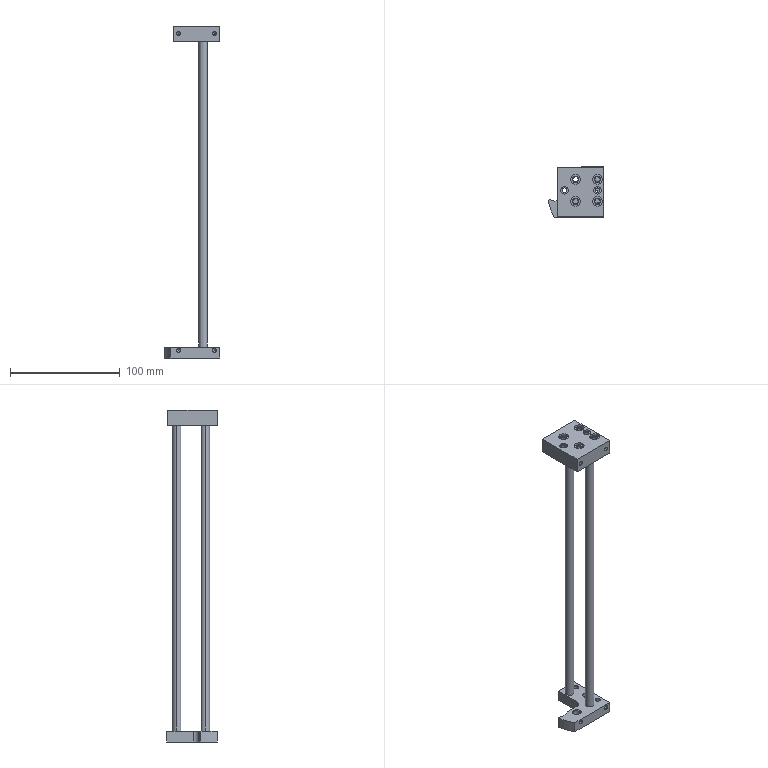Part | STEP file | 1 solid | 172 faces | box 50.109 x 46 x 302 mm | volume 63535 mm3 | cylinder 74 | cone 68 | plane 30 | commonest cylinder face diameters 9 x21 3.2 x14 8 x10 4.8 x8 4 x6 4.5 x4